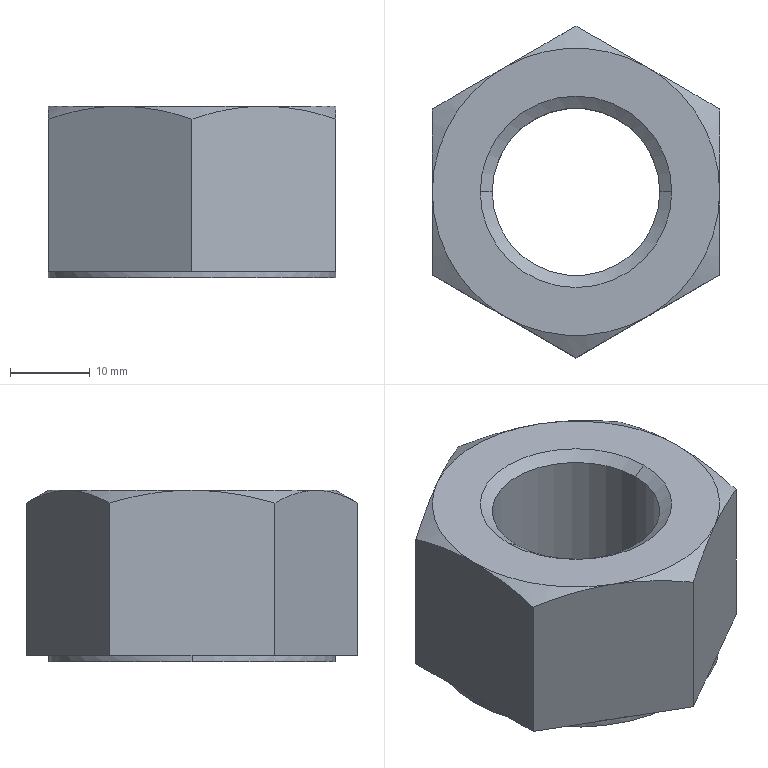Part | STEP file | PN_0069_hex nut-M24x3.0 | 1 solid | 30 faces | box 36 x 41.569 x 21.5 mm | volume 16438 mm3 | plane 14 | cone 10 | cylinder 6 | commonest cylinder face diameters 21 x2 24 x2 36 x2